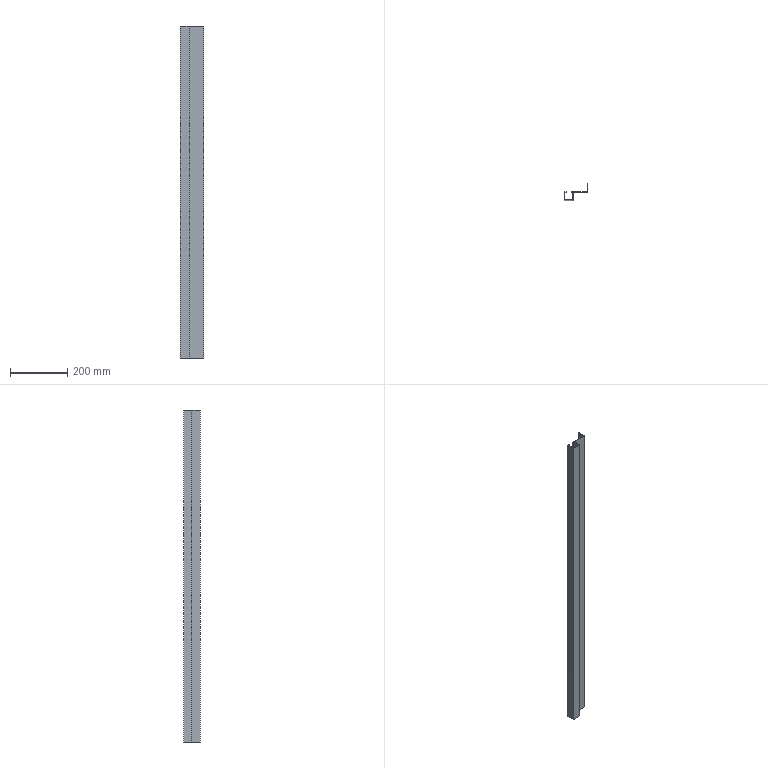Part | STEP file | Rieles_1-21 | 1 solid | 18 faces | box 81.4 x 57.7 x 1164 mm | volume 303280 mm3 | plane 18
STEP:
#1=CARTESIAN_POINT('',(10.,26.2,-712.));
#2=VERTEX_POINT('',#1);
#3=CARTESIAN_POINT('',(10.,27.7,-712.));
#4=VERTEX_POINT('',#3);
#5=CARTESIAN_POINT('',(10.,27.35,-712.));
#6=DIRECTION('',(0.,1.,0.));
#7=VECTOR('',#6,1000.);
#8=LINE('',#5,#7);
#9=EDGE_CURVE('',#2,#4,#8,.T.);
#10=ORIENTED_EDGE('',*,*,#9,.T.);
#11=CARTESIAN_POINT('',(64.2,27.7,-712.));
#12=VERTEX_POINT('',#11);
#13=CARTESIAN_POINT('',(25.,27.7,-712.));
#14=DIRECTION('',(1.,0.,0.));
#15=VECTOR('',#14,1000.);
#16=LINE('',#13,#15);
#17=EDGE_CURVE('',#4,#12,#16,.T.);
#18=ORIENTED_EDGE('',*,*,#17,.T.);
#19=CARTESIAN_POINT('',(64.2,56.2,-712.));
#20=VERTEX_POINT('',#19);
#21=CARTESIAN_POINT('',(64.2,27.35,-712.));
#22=DIRECTION('',(0.,1.,0.));
#23=VECTOR('',#22,1000.);
#24=LINE('',#21,#23);
#25=EDGE_CURVE('',#12,#20,#24,.T.);
#26=ORIENTED_EDGE('',*,*,#25,.T.);
#27=CARTESIAN_POINT('',(65.7,56.2,-712.));
#28=VERTEX_POINT('',#27);
#29=CARTESIAN_POINT('',(25.,56.2,-712.));
#30=DIRECTION('',(1.,0.,0.));
#31=VECTOR('',#30,1000.);
#32=LINE('',#29,#31);
#33=EDGE_CURVE('',#20,#28,#32,.T.);
#34=ORIENTED_EDGE('',*,*,#33,.T.);
#35=CARTESIAN_POINT('',(65.7,26.2,-712.));
#36=VERTEX_POINT('',#35);
#37=CARTESIAN_POINT('',(65.7,27.35,-712.));
#38=DIRECTION('',(0.,-1.,0.));
#39=VECTOR('',#38,1000.);
#40=LINE('',#37,#39);
#41=EDGE_CURVE('',#28,#36,#40,.T.);
#42=ORIENTED_EDGE('',*,*,#41,.T.);
#43=CARTESIAN_POINT('',(15.7,26.2,-712.));
#44=VERTEX_POINT('',#43);
#45=CARTESIAN_POINT('',(25.,26.2,-712.));
#46=DIRECTION('',(-1.,0.,0.));
#47=VECTOR('',#46,1000.);
#48=LINE('',#45,#47);
#49=EDGE_CURVE('',#36,#44,#48,.T.);
#50=ORIENTED_EDGE('',*,*,#49,.T.);
#51=CARTESIAN_POINT('',(15.7,-1.5,-712.));
#52=VERTEX_POINT('',#51);
#53=CARTESIAN_POINT('',(15.7,27.35,-712.));
#54=DIRECTION('',(0.,-1.,0.));
#55=VECTOR('',#54,1000.);
#56=LINE('',#53,#55);
#57=EDGE_CURVE('',#44,#52,#56,.T.);
#58=ORIENTED_EDGE('',*,*,#57,.T.);
#59=CARTESIAN_POINT('',(-15.7,-1.5,-712.));
#60=VERTEX_POINT('',#59);
#61=CARTESIAN_POINT('',(25.,-1.5,-712.));
#62=DIRECTION('',(-1.,0.,0.));
#63=VECTOR('',#62,1000.);
#64=LINE('',#61,#63);
#65=EDGE_CURVE('',#52,#60,#64,.T.);
#66=ORIENTED_EDGE('',*,*,#65,.T.);
#67=CARTESIAN_POINT('',(-15.7,27.7,-712.));
#68=VERTEX_POINT('',#67);
#69=CARTESIAN_POINT('',(-15.7,27.35,-712.));
#70=DIRECTION('',(0.,1.,0.));
#71=VECTOR('',#70,1000.);
#72=LINE('',#69,#71);
#73=EDGE_CURVE('',#60,#68,#72,.T.);
#74=ORIENTED_EDGE('',*,*,#73,.T.);
#75=CARTESIAN_POINT('',(-10.,27.7,-712.));
#76=VERTEX_POINT('',#75);
#77=CARTESIAN_POINT('',(25.,27.7,-712.));
#78=DIRECTION('',(1.,0.,0.));
#79=VECTOR('',#78,1000.);
#80=LINE('',#77,#79);
#81=EDGE_CURVE('',#68,#76,#80,.T.);
#82=ORIENTED_EDGE('',*,*,#81,.T.);
#83=CARTESIAN_POINT('',(-10.,26.2,-712.));
#84=VERTEX_POINT('',#83);
#85=CARTESIAN_POINT('',(-10.,27.35,-712.));
#86=DIRECTION('',(0.,-1.,0.));
#87=VECTOR('',#86,1000.);
#88=LINE('',#85,#87);
#89=EDGE_CURVE('',#76,#84,#88,.T.);
#90=ORIENTED_EDGE('',*,*,#89,.T.);
#91=CARTESIAN_POINT('',(-14.2,26.2,-712.));
#92=VERTEX_POINT('',#91);
#93=CARTESIAN_POINT('',(25.,26.2,-712.));
#94=DIRECTION('',(-1.,0.,0.));
#95=VECTOR('',#94,1000.);
#96=LINE('',#93,#95);
#97=EDGE_CURVE('',#84,#92,#96,.T.);
#98=ORIENTED_EDGE('',*,*,#97,.T.);
#99=CARTESIAN_POINT('',(-14.2,0.,-712.));
#100=VERTEX_POINT('',#99);
#101=CARTESIAN_POINT('',(-14.2,27.35,-712.));
#102=DIRECTION('',(0.,-1.,0.));
#103=VECTOR('',#102,1000.);
#104=LINE('',#101,#103);
#105=EDGE_CURVE('',#92,#100,#104,.T.);
#106=ORIENTED_EDGE('',*,*,#105,.T.);
#107=CARTESIAN_POINT('',(14.2,0.,-712.));
#108=VERTEX_POINT('',#107);
#109=CARTESIAN_POINT('',(25.,0.,-712.));
#110=DIRECTION('',(1.,0.,0.));
#111=VECTOR('',#110,1000.);
#112=LINE('',#109,#111);
#113=EDGE_CURVE('',#100,#108,#112,.T.);
#114=ORIENTED_EDGE('',*,*,#113,.T.);
#115=CARTESIAN_POINT('',(14.2,26.2,-712.));
#116=VERTEX_POINT('',#115);
#117=CARTESIAN_POINT('',(14.2,27.35,-712.));
#118=DIRECTION('',(0.,1.,0.));
#119=VECTOR('',#118,1000.);
#120=LINE('',#117,#119);
#121=EDGE_CURVE('',#108,#116,#120,.T.);
#122=ORIENTED_EDGE('',*,*,#121,.T.);
#123=CARTESIAN_POINT('',(25.,26.2,-712.));
#124=DIRECTION('',(-1.,0.,0.));
#125=VECTOR('',#124,1000.);
#126=LINE('',#123,#125);
#127=EDGE_CURVE('',#116,#2,#126,.T.);
#128=ORIENTED_EDGE('',*,*,#127,.T.);
#129=EDGE_LOOP('',(#10,#18,#26,#34,#42,#50,#58,#66,#74,#82,#90,#98,#106,#114,#122,#128));
#130=FACE_OUTER_BOUND('',#129,.T.);
#131=CARTESIAN_POINT('',(25.,27.35,-712.));
#132=DIRECTION('',(0.,0.,-1.));
#133=DIRECTION('',(0.,-1.,0.));
#134=AXIS2_PLACEMENT_3D('',#131,#132,#133);
#135=PLANE('',#134);
#136=ADVANCED_FACE('',(#130),#135,.T.);
#137=CARTESIAN_POINT('',(10.,26.2,452.));
#138=VERTEX_POINT('',#137);
#139=CARTESIAN_POINT('',(10.,27.7,452.));
#140=VERTEX_POINT('',#139);
#141=CARTESIAN_POINT('',(10.,26.2,452.));
#142=DIRECTION('',(0.,1.,0.));
#143=VECTOR('',#142,1000.);
#144=LINE('',#141,#143);
#145=EDGE_CURVE('',#138,#140,#144,.T.);
#146=ORIENTED_EDGE('',*,*,#145,.F.);
#147=CARTESIAN_POINT('',(14.2,26.2,452.));
#148=VERTEX_POINT('',#147);
#149=CARTESIAN_POINT('',(14.2,26.2,452.));
#150=DIRECTION('',(-1.,0.,0.));
#151=VECTOR('',#150,1000.);
#152=LINE('',#149,#151);
#153=EDGE_CURVE('',#148,#138,#152,.T.);
#154=ORIENTED_EDGE('',*,*,#153,.F.);
#155=CARTESIAN_POINT('',(14.2,0.,452.));
#156=VERTEX_POINT('',#155);
#157=CARTESIAN_POINT('',(14.2,0.,452.));
#158=DIRECTION('',(0.,1.,0.));
#159=VECTOR('',#158,1000.);
#160=LINE('',#157,#159);
#161=EDGE_CURVE('',#156,#148,#160,.T.);
#162=ORIENTED_EDGE('',*,*,#161,.F.);
#163=CARTESIAN_POINT('',(-14.2,0.,452.));
#164=VERTEX_POINT('',#163);
#165=CARTESIAN_POINT('',(-14.2,0.,452.));
#166=DIRECTION('',(1.,0.,0.));
#167=VECTOR('',#166,1000.);
#168=LINE('',#165,#167);
#169=EDGE_CURVE('',#164,#156,#168,.T.);
#170=ORIENTED_EDGE('',*,*,#169,.F.);
#171=CARTESIAN_POINT('',(-14.2,26.2,452.));
#172=VERTEX_POINT('',#171);
#173=CARTESIAN_POINT('',(-14.2,26.2,452.));
#174=DIRECTION('',(0.,-1.,0.));
#175=VECTOR('',#174,1000.);
#176=LINE('',#173,#175);
#177=EDGE_CURVE('',#172,#164,#176,.T.);
#178=ORIENTED_EDGE('',*,*,#177,.F.);
#179=CARTESIAN_POINT('',(-10.,26.2,452.));
#180=VERTEX_POINT('',#179);
#181=CARTESIAN_POINT('',(-10.,26.2,452.));
#182=DIRECTION('',(-1.,0.,0.));
#183=VECTOR('',#182,1000.);
#184=LINE('',#181,#183);
#185=EDGE_CURVE('',#180,#172,#184,.T.);
#186=ORIENTED_EDGE('',*,*,#185,.F.);
#187=CARTESIAN_POINT('',(-10.,27.7,452.));
#188=VERTEX_POINT('',#187);
#189=CARTESIAN_POINT('',(-10.,27.7,452.));
#190=DIRECTION('',(0.,-1.,0.));
#191=VECTOR('',#190,1000.);
#192=LINE('',#189,#191);
#193=EDGE_CURVE('',#188,#180,#192,.T.);
#194=ORIENTED_EDGE('',*,*,#193,.F.);
#195=CARTESIAN_POINT('',(-15.7,27.7,452.));
#196=VERTEX_POINT('',#195);
#197=CARTESIAN_POINT('',(-15.7,27.7,452.));
#198=DIRECTION('',(1.,0.,0.));
#199=VECTOR('',#198,1000.);
#200=LINE('',#197,#199);
#201=EDGE_CURVE('',#196,#188,#200,.T.);
#202=ORIENTED_EDGE('',*,*,#201,.F.);
#203=CARTESIAN_POINT('',(-15.7,-1.5,452.));
#204=VERTEX_POINT('',#203);
#205=CARTESIAN_POINT('',(-15.7,-1.5,452.));
#206=DIRECTION('',(0.,1.,0.));
#207=VECTOR('',#206,1000.);
#208=LINE('',#205,#207);
#209=EDGE_CURVE('',#204,#196,#208,.T.);
#210=ORIENTED_EDGE('',*,*,#209,.F.);
#211=CARTESIAN_POINT('',(15.7,-1.5,452.));
#212=VERTEX_POINT('',#211);
#213=CARTESIAN_POINT('',(15.7,-1.5,452.));
#214=DIRECTION('',(-1.,0.,0.));
#215=VECTOR('',#214,1000.);
#216=LINE('',#213,#215);
#217=EDGE_CURVE('',#212,#204,#216,.T.);
#218=ORIENTED_EDGE('',*,*,#217,.F.);
#219=CARTESIAN_POINT('',(15.7,26.2,452.));
#220=VERTEX_POINT('',#219);
#221=CARTESIAN_POINT('',(15.7,26.2,452.));
#222=DIRECTION('',(0.,-1.,0.));
#223=VECTOR('',#222,1000.);
#224=LINE('',#221,#223);
#225=EDGE_CURVE('',#220,#212,#224,.T.);
#226=ORIENTED_EDGE('',*,*,#225,.F.);
#227=CARTESIAN_POINT('',(65.7,26.2,452.));
#228=VERTEX_POINT('',#227);
#229=CARTESIAN_POINT('',(65.7,26.2,452.));
#230=DIRECTION('',(-1.,0.,0.));
#231=VECTOR('',#230,1000.);
#232=LINE('',#229,#231);
#233=EDGE_CURVE('',#228,#220,#232,.T.);
#234=ORIENTED_EDGE('',*,*,#233,.F.);
#235=CARTESIAN_POINT('',(65.7,56.2,452.));
#236=VERTEX_POINT('',#235);
#237=CARTESIAN_POINT('',(65.7,56.2,452.));
#238=DIRECTION('',(0.,-1.,0.));
#239=VECTOR('',#238,1000.);
#240=LINE('',#237,#239);
#241=EDGE_CURVE('',#236,#228,#240,.T.);
#242=ORIENTED_EDGE('',*,*,#241,.F.);
#243=CARTESIAN_POINT('',(64.2,56.2,452.));
#244=VERTEX_POINT('',#243);
#245=CARTESIAN_POINT('',(64.2,56.2,452.));
#246=DIRECTION('',(1.,0.,0.));
#247=VECTOR('',#246,1000.);
#248=LINE('',#245,#247);
#249=EDGE_CURVE('',#244,#236,#248,.T.);
#250=ORIENTED_EDGE('',*,*,#249,.F.);
#251=CARTESIAN_POINT('',(64.2,27.7,452.));
#252=VERTEX_POINT('',#251);
#253=CARTESIAN_POINT('',(64.2,27.7,452.));
#254=DIRECTION('',(0.,1.,0.));
#255=VECTOR('',#254,1000.);
#256=LINE('',#253,#255);
#257=EDGE_CURVE('',#252,#244,#256,.T.);
#258=ORIENTED_EDGE('',*,*,#257,.F.);
#259=CARTESIAN_POINT('',(10.,27.7,452.));
#260=DIRECTION('',(1.,0.,0.));
#261=VECTOR('',#260,1000.);
#262=LINE('',#259,#261);
#263=EDGE_CURVE('',#140,#252,#262,.T.);
#264=ORIENTED_EDGE('',*,*,#263,.F.);
#265=EDGE_LOOP('',(#146,#154,#162,#170,#178,#186,#194,#202,#210,#218,#226,#234,#242,#250,#258,#264));
#266=FACE_OUTER_BOUND('',#265,.T.);
#267=CARTESIAN_POINT('',(25.,27.35,452.));
#268=DIRECTION('',(0.,0.,1.));
#269=DIRECTION('',(1.,0.,0.));
#270=AXIS2_PLACEMENT_3D('',#267,#268,#269);
#271=PLANE('',#270);
#272=ADVANCED_FACE('',(#266),#271,.T.);
#273=ORIENTED_EDGE('',*,*,#145,.T.);
#274=CARTESIAN_POINT('',(10.,27.7,407.));
#275=DIRECTION('',(0.,0.,-1.));
#276=VECTOR('',#275,1000.);
#277=LINE('',#274,#276);
#278=EDGE_CURVE('',#140,#4,#277,.T.);
#279=ORIENTED_EDGE('',*,*,#278,.T.);
#280=ORIENTED_EDGE('',*,*,#9,.F.);
#281=CARTESIAN_POINT('',(10.,26.2,407.));
#282=DIRECTION('',(0.,0.,-1.));
#283=VECTOR('',#282,1000.);
#284=LINE('',#281,#283);
#285=EDGE_CURVE('',#138,#2,#284,.T.);
#286=ORIENTED_EDGE('',*,*,#285,.F.);
#287=EDGE_LOOP('',(#273,#279,#280,#286));
#288=FACE_OUTER_BOUND('',#287,.T.);
#289=CARTESIAN_POINT('',(10.,26.2,407.));
#290=DIRECTION('',(-1.,0.,0.));
#291=DIRECTION('',(0.,0.,1.));
#292=AXIS2_PLACEMENT_3D('',#289,#290,#291);
#293=PLANE('',#292);
#294=ADVANCED_FACE('',(#288),#293,.T.);
#295=ORIENTED_EDGE('',*,*,#263,.T.);
#296=CARTESIAN_POINT('',(64.2,27.7,407.));
#297=DIRECTION('',(0.,0.,-1.));
#298=VECTOR('',#297,1000.);
#299=LINE('',#296,#298);
#300=EDGE_CURVE('',#252,#12,#299,.T.);
#301=ORIENTED_EDGE('',*,*,#300,.T.);
#302=ORIENTED_EDGE('',*,*,#17,.F.);
#303=ORIENTED_EDGE('',*,*,#278,.F.);
#304=EDGE_LOOP('',(#295,#301,#302,#303));
#305=FACE_OUTER_BOUND('',#304,.T.);
#306=CARTESIAN_POINT('',(10.,27.7,407.));
#307=DIRECTION('',(0.,1.,0.));
#308=DIRECTION('',(1.,0.,0.));
#309=AXIS2_PLACEMENT_3D('',#306,#307,#308);
#310=PLANE('',#309);
#311=ADVANCED_FACE('',(#305),#310,.T.);
#312=ORIENTED_EDGE('',*,*,#257,.T.);
#313=CARTESIAN_POINT('',(64.2,56.2,407.));
#314=DIRECTION('',(0.,0.,-1.));
#315=VECTOR('',#314,1000.);
#316=LINE('',#313,#315);
#317=EDGE_CURVE('',#244,#20,#316,.T.);
#318=ORIENTED_EDGE('',*,*,#317,.T.);
#319=ORIENTED_EDGE('',*,*,#25,.F.);
#320=ORIENTED_EDGE('',*,*,#300,.F.);
#321=EDGE_LOOP('',(#312,#318,#319,#320));
#322=FACE_OUTER_BOUND('',#321,.T.);
#323=CARTESIAN_POINT('',(64.2,27.7,407.));
#324=DIRECTION('',(-1.,0.,0.));
#325=DIRECTION('',(0.,0.,1.));
#326=AXIS2_PLACEMENT_3D('',#323,#324,#325);
#327=PLANE('',#326);
#328=ADVANCED_FACE('',(#322),#327,.T.);
#329=ORIENTED_EDGE('',*,*,#249,.T.);
#330=CARTESIAN_POINT('',(65.7,56.2,407.));
#331=DIRECTION('',(0.,0.,-1.));
#332=VECTOR('',#331,1000.);
#333=LINE('',#330,#332);
#334=EDGE_CURVE('',#236,#28,#333,.T.);
#335=ORIENTED_EDGE('',*,*,#334,.T.);
#336=ORIENTED_EDGE('',*,*,#33,.F.);
#337=ORIENTED_EDGE('',*,*,#317,.F.);
#338=EDGE_LOOP('',(#329,#335,#336,#337));
#339=FACE_OUTER_BOUND('',#338,.T.);
#340=CARTESIAN_POINT('',(64.2,56.2,407.));
#341=DIRECTION('',(0.,1.,0.));
#342=DIRECTION('',(1.,0.,0.));
#343=AXIS2_PLACEMENT_3D('',#340,#341,#342);
#344=PLANE('',#343);
#345=ADVANCED_FACE('',(#339),#344,.T.);
#346=ORIENTED_EDGE('',*,*,#241,.T.);
#347=CARTESIAN_POINT('',(65.7,26.2,407.));
#348=DIRECTION('',(0.,0.,-1.));
#349=VECTOR('',#348,1000.);
#350=LINE('',#347,#349);
#351=EDGE_CURVE('',#228,#36,#350,.T.);
#352=ORIENTED_EDGE('',*,*,#351,.T.);
#353=ORIENTED_EDGE('',*,*,#41,.F.);
#354=ORIENTED_EDGE('',*,*,#334,.F.);
#355=EDGE_LOOP('',(#346,#352,#353,#354));
#356=FACE_OUTER_BOUND('',#355,.T.);
#357=CARTESIAN_POINT('',(65.7,56.2,407.));
#358=DIRECTION('',(1.,0.,0.));
#359=DIRECTION('',(0.,-1.,0.));
#360=AXIS2_PLACEMENT_3D('',#357,#358,#359);
#361=PLANE('',#360);
#362=ADVANCED_FACE('',(#356),#361,.T.);
#363=ORIENTED_EDGE('',*,*,#233,.T.);
#364=CARTESIAN_POINT('',(15.7,26.2,407.));
#365=DIRECTION('',(0.,0.,-1.));
#366=VECTOR('',#365,1000.);
#367=LINE('',#364,#366);
#368=EDGE_CURVE('',#220,#44,#367,.T.);
#369=ORIENTED_EDGE('',*,*,#368,.T.);
#370=ORIENTED_EDGE('',*,*,#49,.F.);
#371=ORIENTED_EDGE('',*,*,#351,.F.);
#372=EDGE_LOOP('',(#363,#369,#370,#371));
#373=FACE_OUTER_BOUND('',#372,.T.);
#374=CARTESIAN_POINT('',(65.7,26.2,407.));
#375=DIRECTION('',(0.,-1.,0.));
#376=DIRECTION('',(0.,0.,-1.));
#377=AXIS2_PLACEMENT_3D('',#374,#375,#376);
#378=PLANE('',#377);
#379=ADVANCED_FACE('',(#373),#378,.T.);
#380=ORIENTED_EDGE('',*,*,#225,.T.);
#381=CARTESIAN_POINT('',(15.7,-1.5,407.));
#382=DIRECTION('',(0.,0.,-1.));
#383=VECTOR('',#382,1000.);
#384=LINE('',#381,#383);
#385=EDGE_CURVE('',#212,#52,#384,.T.);
#386=ORIENTED_EDGE('',*,*,#385,.T.);
#387=ORIENTED_EDGE('',*,*,#57,.F.);
#388=ORIENTED_EDGE('',*,*,#368,.F.);
#389=EDGE_LOOP('',(#380,#386,#387,#388));
#390=FACE_OUTER_BOUND('',#389,.T.);
#391=CARTESIAN_POINT('',(15.7,26.2,407.));
#392=DIRECTION('',(1.,0.,0.));
#393=DIRECTION('',(0.,1.,0.));
#394=AXIS2_PLACEMENT_3D('',#391,#392,#393);
#395=PLANE('',#394);
#396=ADVANCED_FACE('',(#390),#395,.T.);
#397=ORIENTED_EDGE('',*,*,#217,.T.);
#398=CARTESIAN_POINT('',(-15.7,-1.5,407.));
#399=DIRECTION('',(0.,0.,-1.));
#400=VECTOR('',#399,1000.);
#401=LINE('',#398,#400);
#402=EDGE_CURVE('',#204,#60,#401,.T.);
#403=ORIENTED_EDGE('',*,*,#402,.T.);
#404=ORIENTED_EDGE('',*,*,#65,.F.);
#405=ORIENTED_EDGE('',*,*,#385,.F.);
#406=EDGE_LOOP('',(#397,#403,#404,#405));
#407=FACE_OUTER_BOUND('',#406,.T.);
#408=CARTESIAN_POINT('',(15.7,-1.5,407.));
#409=DIRECTION('',(0.,-1.,0.));
#410=DIRECTION('',(0.,0.,-1.));
#411=AXIS2_PLACEMENT_3D('',#408,#409,#410);
#412=PLANE('',#411);
#413=ADVANCED_FACE('',(#407),#412,.T.);
#414=ORIENTED_EDGE('',*,*,#209,.T.);
#415=CARTESIAN_POINT('',(-15.7,27.7,407.));
#416=DIRECTION('',(0.,0.,-1.));
#417=VECTOR('',#416,1000.);
#418=LINE('',#415,#417);
#419=EDGE_CURVE('',#196,#68,#418,.T.);
#420=ORIENTED_EDGE('',*,*,#419,.T.);
#421=ORIENTED_EDGE('',*,*,#73,.F.);
#422=ORIENTED_EDGE('',*,*,#402,.F.);
#423=EDGE_LOOP('',(#414,#420,#421,#422));
#424=FACE_OUTER_BOUND('',#423,.T.);
#425=CARTESIAN_POINT('',(-15.7,-1.5,407.));
#426=DIRECTION('',(-1.,0.,0.));
#427=DIRECTION('',(0.,0.,1.));
#428=AXIS2_PLACEMENT_3D('',#425,#426,#427);
#429=PLANE('',#428);
#430=ADVANCED_FACE('',(#424),#429,.T.);
#431=ORIENTED_EDGE('',*,*,#201,.T.);
#432=CARTESIAN_POINT('',(-10.,27.7,407.));
#433=DIRECTION('',(0.,0.,-1.));
#434=VECTOR('',#433,1000.);
#435=LINE('',#432,#434);
#436=EDGE_CURVE('',#188,#76,#435,.T.);
#437=ORIENTED_EDGE('',*,*,#436,.T.);
#438=ORIENTED_EDGE('',*,*,#81,.F.);
#439=ORIENTED_EDGE('',*,*,#419,.F.);
#440=EDGE_LOOP('',(#431,#437,#438,#439));
#441=FACE_OUTER_BOUND('',#440,.T.);
#442=CARTESIAN_POINT('',(-15.7,27.7,407.));
#443=DIRECTION('',(0.,1.,0.));
#444=DIRECTION('',(1.,0.,0.));
#445=AXIS2_PLACEMENT_3D('',#442,#443,#444);
#446=PLANE('',#445);
#447=ADVANCED_FACE('',(#441),#446,.T.);
#448=ORIENTED_EDGE('',*,*,#193,.T.);
#449=CARTESIAN_POINT('',(-10.,26.2,407.));
#450=DIRECTION('',(0.,0.,-1.));
#451=VECTOR('',#450,1000.);
#452=LINE('',#449,#451);
#453=EDGE_CURVE('',#180,#84,#452,.T.);
#454=ORIENTED_EDGE('',*,*,#453,.T.);
#455=ORIENTED_EDGE('',*,*,#89,.F.);
#456=ORIENTED_EDGE('',*,*,#436,.F.);
#457=EDGE_LOOP('',(#448,#454,#455,#456));
#458=FACE_OUTER_BOUND('',#457,.T.);
#459=CARTESIAN_POINT('',(-10.,27.7,407.));
#460=DIRECTION('',(1.,0.,0.));
#461=DIRECTION('',(0.,1.,0.));
#462=AXIS2_PLACEMENT_3D('',#459,#460,#461);
#463=PLANE('',#462);
#464=ADVANCED_FACE('',(#458),#463,.T.);
#465=ORIENTED_EDGE('',*,*,#185,.T.);
#466=CARTESIAN_POINT('',(-14.2,26.2,407.));
#467=DIRECTION('',(0.,0.,-1.));
#468=VECTOR('',#467,1000.);
#469=LINE('',#466,#468);
#470=EDGE_CURVE('',#172,#92,#469,.T.);
#471=ORIENTED_EDGE('',*,*,#470,.T.);
#472=ORIENTED_EDGE('',*,*,#97,.F.);
#473=ORIENTED_EDGE('',*,*,#453,.F.);
#474=EDGE_LOOP('',(#465,#471,#472,#473));
#475=FACE_OUTER_BOUND('',#474,.T.);
#476=CARTESIAN_POINT('',(-10.,26.2,407.));
#477=DIRECTION('',(0.,-1.,0.));
#478=DIRECTION('',(0.,0.,-1.));
#479=AXIS2_PLACEMENT_3D('',#476,#477,#478);
#480=PLANE('',#479);
#481=ADVANCED_FACE('',(#475),#480,.T.);
#482=ORIENTED_EDGE('',*,*,#177,.T.);
#483=CARTESIAN_POINT('',(-14.2,0.,407.));
#484=DIRECTION('',(0.,0.,-1.));
#485=VECTOR('',#484,1000.);
#486=LINE('',#483,#485);
#487=EDGE_CURVE('',#164,#100,#486,.T.);
#488=ORIENTED_EDGE('',*,*,#487,.T.);
#489=ORIENTED_EDGE('',*,*,#105,.F.);
#490=ORIENTED_EDGE('',*,*,#470,.F.);
#491=EDGE_LOOP('',(#482,#488,#489,#490));
#492=FACE_OUTER_BOUND('',#491,.T.);
#493=CARTESIAN_POINT('',(-14.2,26.2,407.));
#494=DIRECTION('',(1.,0.,0.));
#495=DIRECTION('',(0.,1.,0.));
#496=AXIS2_PLACEMENT_3D('',#493,#494,#495);
#497=PLANE('',#496);
#498=ADVANCED_FACE('',(#492),#497,.T.);
#499=ORIENTED_EDGE('',*,*,#169,.T.);
#500=CARTESIAN_POINT('',(14.2,0.,407.));
#501=DIRECTION('',(0.,0.,-1.));
#502=VECTOR('',#501,1000.);
#503=LINE('',#500,#502);
#504=EDGE_CURVE('',#156,#108,#503,.T.);
#505=ORIENTED_EDGE('',*,*,#504,.T.);
#506=ORIENTED_EDGE('',*,*,#113,.F.);
#507=ORIENTED_EDGE('',*,*,#487,.F.);
#508=EDGE_LOOP('',(#499,#505,#506,#507));
#509=FACE_OUTER_BOUND('',#508,.T.);
#510=CARTESIAN_POINT('',(-14.2,0.,407.));
#511=DIRECTION('',(0.,1.,0.));
#512=DIRECTION('',(1.,0.,0.));
#513=AXIS2_PLACEMENT_3D('',#510,#511,#512);
#514=PLANE('',#513);
#515=ADVANCED_FACE('',(#509),#514,.T.);
#516=ORIENTED_EDGE('',*,*,#161,.T.);
#517=CARTESIAN_POINT('',(14.2,26.2,407.));
#518=DIRECTION('',(0.,0.,-1.));
#519=VECTOR('',#518,1000.);
#520=LINE('',#517,#519);
#521=EDGE_CURVE('',#148,#116,#520,.T.);
#522=ORIENTED_EDGE('',*,*,#521,.T.);
#523=ORIENTED_EDGE('',*,*,#121,.F.);
#524=ORIENTED_EDGE('',*,*,#504,.F.);
#525=EDGE_LOOP('',(#516,#522,#523,#524));
#526=FACE_OUTER_BOUND('',#525,.T.);
#527=CARTESIAN_POINT('',(14.2,0.,407.));
#528=DIRECTION('',(-1.,0.,0.));
#529=DIRECTION('',(0.,0.,1.));
#530=AXIS2_PLACEMENT_3D('',#527,#528,#529);
#531=PLANE('',#530);
#532=ADVANCED_FACE('',(#526),#531,.T.);
#533=ORIENTED_EDGE('',*,*,#153,.T.);
#534=ORIENTED_EDGE('',*,*,#285,.T.);
#535=ORIENTED_EDGE('',*,*,#127,.F.);
#536=ORIENTED_EDGE('',*,*,#521,.F.);
#537=EDGE_LOOP('',(#533,#534,#535,#536));
#538=FACE_OUTER_BOUND('',#537,.T.);
#539=CARTESIAN_POINT('',(14.2,26.2,407.));
#540=DIRECTION('',(0.,-1.,0.));
#541=DIRECTION('',(-1.,0.,0.));
#542=AXIS2_PLACEMENT_3D('',#539,#540,#541);
#543=PLANE('',#542);
#544=ADVANCED_FACE('',(#538),#543,.T.);
#545=CLOSED_SHELL('',(#136,#272,#294,#311,#328,#345,#362,#379,#396,#413,#430,#447,#464,#481,#498,#515,#532,#544));
#546=MANIFOLD_SOLID_BREP('',#545);
#547=CARTESIAN_POINT('',(0.,0.,0.));
#548=DIRECTION('',(0.,0.,1.));
#549=DIRECTION('',(1.,0.,0.));
#550=AXIS2_PLACEMENT_3D('',#547,#548,#549);
#551=(LENGTH_UNIT()NAMED_UNIT(*)SI_UNIT(.MILLI.,.METRE.));
#552=UNCERTAINTY_MEASURE_WITH_UNIT(LENGTH_MEASURE(0.00001),#551,'','');
#553=(NAMED_UNIT(*)PLANE_ANGLE_UNIT()SI_UNIT($,.RADIAN.));
#554=(NAMED_UNIT(*)SI_UNIT($,.STERADIAN.)SOLID_ANGLE_UNIT());
#555=(GEOMETRIC_REPRESENTATION_CONTEXT(3)GLOBAL_UNCERTAINTY_ASSIGNED_CONTEXT((#552))GLOBAL_UNIT_ASSIGNED_CONTEXT((#551,#553,#554))REPRESENTATION_CONTEXT('',''));
#556=ADVANCED_BREP_SHAPE_REPRESENTATION('',(#546,#550),#555);